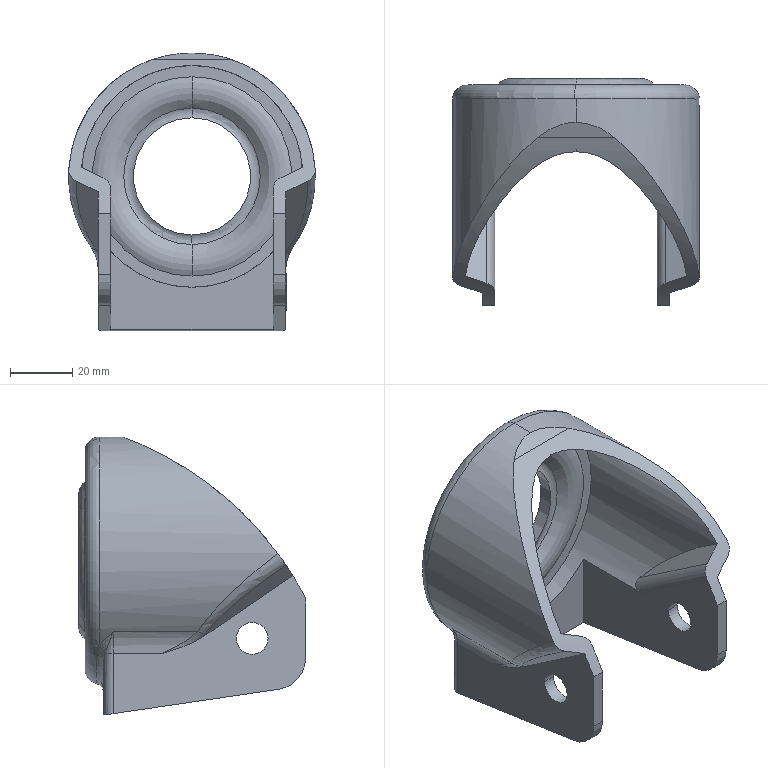Part | NX | features solid 2 | 1 solid | 123 faces | box 79 x 72.7 x 89 mm | volume 59884 mm3 | plane 54 | cylinder 33 | spline 19 | torus 17 | commonest cylinder face diameters 10.2 x4 2.7 x3 6.56 x3 6 x2 6.8 x2 10 x2